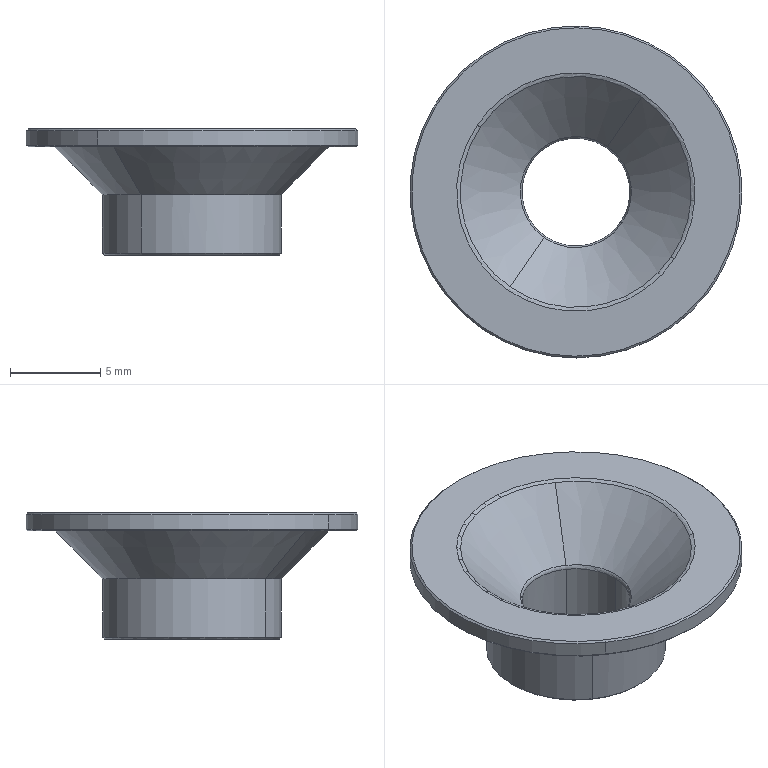Part | SolidWorks | features BaseBody 1 | 1 solid | 30 faces | box 18.44 x 18.44 x 7 mm | volume 502.721 mm3 | cone 14 | cylinder 9 | torus 4 | plane 3 | commonest cylinder face diameters 6 x3 9.94 x3 18.44 x3
STEP:
#1=CARTESIAN_POINT('',(96.116,-202.239,3.349));
#2=VERTEX_POINT('',#1);
#3=CARTESIAN_POINT('',(96.116,-202.239,0.1));
#4=VERTEX_POINT('',#3);
#5=CARTESIAN_POINT('',(96.116,-202.239,2.124));
#6=DIRECTION('',(0.,0.,-1.));
#7=VECTOR('',#6,1000.);
#8=LINE('',#5,#7);
#9=EDGE_CURVE('',#2,#4,#8,.T.);
#10=ORIENTED_EDGE('',*,*,#9,.F.);
#11=CARTESIAN_POINT('',(88.325,-206.142,3.349));
#12=VERTEX_POINT('',#11);
#13=CARTESIAN_POINT('',(91.15,-202.053,3.349));
#14=DIRECTION('',(0.,0.,-1.));
#15=DIRECTION('',(0.5684,0.8228,0.));
#16=AXIS2_PLACEMENT_3D('',#13,#14,#15);
#17=CIRCLE('',#16,4.97);
#18=EDGE_CURVE('',#2,#12,#17,.T.);
#19=ORIENTED_EDGE('',*,*,#18,.T.);
#20=CARTESIAN_POINT('',(88.325,-206.142,0.1));
#21=VERTEX_POINT('',#20);
#22=CARTESIAN_POINT('',(88.325,-206.142,0.1));
#23=DIRECTION('',(0.,0.,1.));
#24=VECTOR('',#23,1000.);
#25=LINE('',#22,#24);
#26=EDGE_CURVE('',#21,#12,#25,.T.);
#27=ORIENTED_EDGE('',*,*,#26,.F.);
#28=CARTESIAN_POINT('',(90.964,-207.019,0.1));
#29=VERTEX_POINT('',#28);
#30=CARTESIAN_POINT('',(91.15,-202.053,0.1));
#31=DIRECTION('',(0.,0.,1.));
#32=DIRECTION('',(-0.5684,-0.8228,0.));
#33=AXIS2_PLACEMENT_3D('',#30,#31,#32);
#34=CIRCLE('',#33,4.97);
#35=EDGE_CURVE('',#21,#29,#34,.T.);
#36=ORIENTED_EDGE('',*,*,#35,.T.);
#37=CARTESIAN_POINT('',(91.15,-202.053,0.1));
#38=DIRECTION('',(0.,0.,1.));
#39=DIRECTION('',(-0.5684,-0.8228,0.));
#40=AXIS2_PLACEMENT_3D('',#37,#38,#39);
#41=CIRCLE('',#40,4.97);
#42=EDGE_CURVE('',#29,#4,#41,.T.);
#43=ORIENTED_EDGE('',*,*,#42,.T.);
#44=EDGE_LOOP('',(#10,#19,#27,#36,#43));
#45=FACE_OUTER_BOUND('',#44,.T.);
#46=CARTESIAN_POINT('',(91.15,-202.053,2.124));
#47=DIRECTION('',(0.,0.,-1.));
#48=DIRECTION('',(0.9993,-0.03741,0.));
#49=AXIS2_PLACEMENT_3D('',#46,#47,#48);
#50=CYLINDRICAL_SURFACE('',#49,4.97);
#51=ADVANCED_FACE('',(#45),#50,.T.);
#52=CARTESIAN_POINT('',(90.967,-206.919,0.));
#53=VERTEX_POINT('',#52);
#54=CARTESIAN_POINT('',(90.966,-206.969,0.05));
#55=DIRECTION('',(-0.02645,-0.7066,0.7071));
#56=VECTOR('',#55,1000.);
#57=LINE('',#54,#56);
#58=EDGE_CURVE('',#53,#29,#57,.T.);
#59=ORIENTED_EDGE('',*,*,#58,.F.);
#60=CARTESIAN_POINT('',(93.918,-198.046,0.));
#61=VERTEX_POINT('',#60);
#62=CARTESIAN_POINT('',(91.15,-202.053,0.));
#63=DIRECTION('',(0.,0.,1.));
#64=DIRECTION('',(-0.5684,-0.8228,0.));
#65=AXIS2_PLACEMENT_3D('',#62,#63,#64);
#66=CIRCLE('',#65,4.87);
#67=EDGE_CURVE('',#53,#61,#66,.T.);
#68=ORIENTED_EDGE('',*,*,#67,.T.);
#69=CARTESIAN_POINT('',(93.974,-197.964,0.1));
#70=VERTEX_POINT('',#69);
#71=CARTESIAN_POINT('',(93.974,-197.964,0.1));
#72=DIRECTION('',(-0.4019,-0.5818,-0.7071));
#73=VECTOR('',#72,1000.);
#74=LINE('',#71,#73);
#75=EDGE_CURVE('',#70,#61,#74,.T.);
#76=ORIENTED_EDGE('',*,*,#75,.F.);
#77=CARTESIAN_POINT('',(91.15,-202.053,0.1));
#78=DIRECTION('',(0.,0.,1.));
#79=DIRECTION('',(-0.5684,-0.8228,0.));
#80=AXIS2_PLACEMENT_3D('',#77,#78,#79);
#81=CIRCLE('',#80,4.97);
#82=EDGE_CURVE('',#4,#70,#81,.T.);
#83=ORIENTED_EDGE('',*,*,#82,.F.);
#84=ORIENTED_EDGE('',*,*,#42,.F.);
#85=EDGE_LOOP('',(#59,#68,#76,#83,#84));
#86=FACE_OUTER_BOUND('',#85,.T.);
#87=CARTESIAN_POINT('',(91.15,-202.053,0.05));
#88=DIRECTION('',(0.,0.,1.));
#89=DIRECTION('',(-0.03741,-0.9993,0.));
#90=AXIS2_PLACEMENT_3D('',#87,#88,#89);
#91=CONICAL_SURFACE('',#90,4.92,0.7854);
#92=ADVANCED_FACE('',(#86),#91,.T.);
#93=ORIENTED_EDGE('',*,*,#75,.T.);
#94=CARTESIAN_POINT('',(88.382,-206.06,0.));
#95=VERTEX_POINT('',#94);
#96=CARTESIAN_POINT('',(91.15,-202.053,0.));
#97=DIRECTION('',(0.,0.,1.));
#98=DIRECTION('',(0.5684,0.8228,0.));
#99=AXIS2_PLACEMENT_3D('',#96,#97,#98);
#100=CIRCLE('',#99,4.87);
#101=EDGE_CURVE('',#61,#95,#100,.T.);
#102=ORIENTED_EDGE('',*,*,#101,.T.);
#103=CARTESIAN_POINT('',(88.325,-206.142,0.1));
#104=DIRECTION('',(0.4019,0.5818,-0.7071));
#105=VECTOR('',#104,1000.);
#106=LINE('',#103,#105);
#107=EDGE_CURVE('',#21,#95,#106,.T.);
#108=ORIENTED_EDGE('',*,*,#107,.F.);
#109=CARTESIAN_POINT('',(91.15,-202.053,0.1));
#110=DIRECTION('',(0.,0.,1.));
#111=DIRECTION('',(-0.9993,0.03741,0.));
#112=AXIS2_PLACEMENT_3D('',#109,#110,#111);
#113=CIRCLE('',#112,4.97);
#114=EDGE_CURVE('',#70,#21,#113,.T.);
#115=ORIENTED_EDGE('',*,*,#114,.F.);
#116=EDGE_LOOP('',(#93,#102,#108,#115));
#117=FACE_OUTER_BOUND('',#116,.T.);
#118=CARTESIAN_POINT('',(91.15,-202.053,0.05));
#119=DIRECTION('',(0.,0.,1.));
#120=DIRECTION('',(-0.03741,-0.9993,0.));
#121=AXIS2_PLACEMENT_3D('',#118,#119,#120);
#122=CONICAL_SURFACE('',#121,4.92,0.7854);
#123=ADVANCED_FACE('',(#117),#122,.T.);
#124=ORIENTED_EDGE('',*,*,#26,.T.);
#125=CARTESIAN_POINT('',(93.974,-197.964,3.349));
#126=VERTEX_POINT('',#125);
#127=CARTESIAN_POINT('',(91.15,-202.053,3.349));
#128=DIRECTION('',(0.,0.,-1.));
#129=DIRECTION('',(-0.5684,-0.8228,0.));
#130=AXIS2_PLACEMENT_3D('',#127,#128,#129);
#131=CIRCLE('',#130,4.97);
#132=EDGE_CURVE('',#12,#126,#131,.T.);
#133=ORIENTED_EDGE('',*,*,#132,.T.);
#134=CARTESIAN_POINT('',(93.974,-197.964,3.349));
#135=DIRECTION('',(0.,0.,-1.));
#136=VECTOR('',#135,1000.);
#137=LINE('',#134,#136);
#138=EDGE_CURVE('',#126,#70,#137,.T.);
#139=ORIENTED_EDGE('',*,*,#138,.T.);
#140=ORIENTED_EDGE('',*,*,#114,.T.);
#141=EDGE_LOOP('',(#124,#133,#139,#140));
#142=FACE_OUTER_BOUND('',#141,.T.);
#143=CARTESIAN_POINT('',(91.15,-202.053,2.124));
#144=DIRECTION('',(0.,0.,-1.));
#145=DIRECTION('',(0.9993,-0.03741,0.));
#146=AXIS2_PLACEMENT_3D('',#143,#144,#145);
#147=CYLINDRICAL_SURFACE('',#146,4.97);
#148=ADVANCED_FACE('',(#142),#147,.T.);
#149=CARTESIAN_POINT('',(86.818,-208.323,6.));
#150=VERTEX_POINT('',#149);
#151=CARTESIAN_POINT('',(88.325,-206.142,3.349));
#152=DIRECTION('',(-0.4019,-0.5818,0.7071));
#153=VECTOR('',#152,1000.);
#154=LINE('',#151,#153);
#155=EDGE_CURVE('',#12,#150,#154,.T.);
#156=ORIENTED_EDGE('',*,*,#155,.T.);
#157=CARTESIAN_POINT('',(95.481,-195.782,6.));
#158=VERTEX_POINT('',#157);
#159=CARTESIAN_POINT('',(91.15,-202.053,6.));
#160=DIRECTION('',(0.,0.,-1.));
#161=DIRECTION('',(-0.5684,-0.8228,0.));
#162=AXIS2_PLACEMENT_3D('',#159,#160,#161);
#163=CIRCLE('',#162,7.621);
#164=EDGE_CURVE('',#150,#158,#163,.T.);
#165=ORIENTED_EDGE('',*,*,#164,.T.);
#166=CARTESIAN_POINT('',(95.481,-195.782,6.));
#167=DIRECTION('',(-0.4019,-0.5818,-0.7071));
#168=VECTOR('',#167,1000.);
#169=LINE('',#166,#168);
#170=EDGE_CURVE('',#158,#126,#169,.T.);
#171=ORIENTED_EDGE('',*,*,#170,.T.);
#172=ORIENTED_EDGE('',*,*,#132,.F.);
#173=EDGE_LOOP('',(#156,#165,#171,#172));
#174=FACE_OUTER_BOUND('',#173,.T.);
#175=CARTESIAN_POINT('',(91.15,-202.053,4.674));
#176=DIRECTION('',(0.,0.,1.));
#177=DIRECTION('',(0.8228,-0.5684,0.));
#178=AXIS2_PLACEMENT_3D('',#175,#176,#177);
#179=CONICAL_SURFACE('',#178,6.296,0.7854);
#180=ADVANCED_FACE('',(#174),#179,.T.);
#181=ORIENTED_EDGE('',*,*,#155,.F.);
#182=ORIENTED_EDGE('',*,*,#18,.F.);
#183=CARTESIAN_POINT('',(91.15,-202.053,3.349));
#184=DIRECTION('',(0.,0.,-1.));
#185=DIRECTION('',(0.5684,0.8228,0.));
#186=AXIS2_PLACEMENT_3D('',#183,#184,#185);
#187=CIRCLE('',#186,4.97);
#188=EDGE_CURVE('',#126,#2,#187,.T.);
#189=ORIENTED_EDGE('',*,*,#188,.F.);
#190=ORIENTED_EDGE('',*,*,#170,.F.);
#191=CARTESIAN_POINT('',(91.15,-202.053,6.));
#192=DIRECTION('',(0.,0.,-1.));
#193=DIRECTION('',(0.5684,0.8228,0.));
#194=AXIS2_PLACEMENT_3D('',#191,#192,#193);
#195=CIRCLE('',#194,7.621);
#196=EDGE_CURVE('',#158,#150,#195,.T.);
#197=ORIENTED_EDGE('',*,*,#196,.T.);
#198=EDGE_LOOP('',(#181,#182,#189,#190,#197));
#199=FACE_OUTER_BOUND('',#198,.T.);
#200=CARTESIAN_POINT('',(91.15,-202.053,4.674));
#201=DIRECTION('',(0.,0.,1.));
#202=DIRECTION('',(-0.8228,0.5684,0.));
#203=AXIS2_PLACEMENT_3D('',#200,#201,#202);
#204=CONICAL_SURFACE('',#203,6.296,0.7854);
#205=ADVANCED_FACE('',(#199),#204,.T.);
#206=ORIENTED_EDGE('',*,*,#164,.F.);
#207=ORIENTED_EDGE('',*,*,#196,.F.);
#208=EDGE_LOOP('',(#206,#207));
#209=FACE_BOUND('',#208,.T.);
#210=CARTESIAN_POINT('',(85.966,-209.556,6.));
#211=VERTEX_POINT('',#210);
#212=CARTESIAN_POINT('',(96.333,-194.549,6.));
#213=VERTEX_POINT('',#212);
#214=CARTESIAN_POINT('',(91.15,-202.053,6.));
#215=DIRECTION('',(0.,0.,1.));
#216=DIRECTION('',(-0.5684,-0.8228,0.));
#217=AXIS2_PLACEMENT_3D('',#214,#215,#216);
#218=CIRCLE('',#217,9.12);
#219=EDGE_CURVE('',#211,#213,#218,.T.);
#220=ORIENTED_EDGE('',*,*,#219,.F.);
#221=CARTESIAN_POINT('',(91.15,-202.053,6.));
#222=DIRECTION('',(0.,0.,1.));
#223=DIRECTION('',(-0.8228,0.5684,0.));
#224=AXIS2_PLACEMENT_3D('',#221,#222,#223);
#225=CIRCLE('',#224,9.12);
#226=EDGE_CURVE('',#213,#211,#225,.T.);
#227=ORIENTED_EDGE('',*,*,#226,.F.);
#228=EDGE_LOOP('',(#220,#227));
#229=FACE_OUTER_BOUND('',#228,.T.);
#230=CARTESIAN_POINT('',(106.374,-199.269,6.));
#231=DIRECTION('',(0.,0.,-1.));
#232=DIRECTION('',(0.,-1.,0.));
#233=AXIS2_PLACEMENT_3D('',#230,#231,#232);
#234=PLANE('',#233);
#235=ADVANCED_FACE('',(#209,#229),#234,.T.);
#236=ORIENTED_EDGE('',*,*,#219,.T.);
#237=CARTESIAN_POINT('',(96.39,-194.467,6.1));
#238=VERTEX_POINT('',#237);
#239=CARTESIAN_POINT('',(96.39,-194.467,6.1));
#240=DIRECTION('',(-0.4019,-0.5818,-0.7071));
#241=VECTOR('',#240,1000.);
#242=LINE('',#239,#241);
#243=EDGE_CURVE('',#238,#213,#242,.T.);
#244=ORIENTED_EDGE('',*,*,#243,.F.);
#245=CARTESIAN_POINT('',(100.363,-202.398,6.1));
#246=VERTEX_POINT('',#245);
#247=CARTESIAN_POINT('',(91.15,-202.053,6.1));
#248=DIRECTION('',(0.,0.,1.));
#249=DIRECTION('',(0.9993,-0.03741,0.));
#250=AXIS2_PLACEMENT_3D('',#247,#248,#249);
#251=CIRCLE('',#250,9.22);
#252=EDGE_CURVE('',#246,#238,#251,.T.);
#253=ORIENTED_EDGE('',*,*,#252,.F.);
#254=CARTESIAN_POINT('',(85.909,-209.639,6.1));
#255=VERTEX_POINT('',#254);
#256=CARTESIAN_POINT('',(91.15,-202.053,6.1));
#257=DIRECTION('',(0.,0.,1.));
#258=DIRECTION('',(0.9993,-0.03741,0.));
#259=AXIS2_PLACEMENT_3D('',#256,#257,#258);
#260=CIRCLE('',#259,9.22);
#261=EDGE_CURVE('',#255,#246,#260,.T.);
#262=ORIENTED_EDGE('',*,*,#261,.F.);
#263=CARTESIAN_POINT('',(85.966,-209.556,6.));
#264=DIRECTION('',(-0.4019,-0.5818,0.7071));
#265=VECTOR('',#264,1000.);
#266=LINE('',#263,#265);
#267=EDGE_CURVE('',#211,#255,#266,.T.);
#268=ORIENTED_EDGE('',*,*,#267,.F.);
#269=EDGE_LOOP('',(#236,#244,#253,#262,#268));
#270=FACE_OUTER_BOUND('',#269,.T.);
#271=CARTESIAN_POINT('',(91.15,-202.053,6.05));
#272=DIRECTION('',(0.,0.,1.));
#273=DIRECTION('',(-0.8228,0.5684,0.));
#274=AXIS2_PLACEMENT_3D('',#271,#272,#273);
#275=CONICAL_SURFACE('',#274,9.17,0.7854);
#276=ADVANCED_FACE('',(#270),#275,.T.);
#277=ORIENTED_EDGE('',*,*,#226,.T.);
#278=ORIENTED_EDGE('',*,*,#267,.T.);
#279=CARTESIAN_POINT('',(91.15,-202.053,6.1));
#280=DIRECTION('',(0.,0.,1.));
#281=DIRECTION('',(-0.9993,0.03741,0.));
#282=AXIS2_PLACEMENT_3D('',#279,#280,#281);
#283=CIRCLE('',#282,9.22);
#284=EDGE_CURVE('',#238,#255,#283,.T.);
#285=ORIENTED_EDGE('',*,*,#284,.F.);
#286=ORIENTED_EDGE('',*,*,#243,.T.);
#287=EDGE_LOOP('',(#277,#278,#285,#286));
#288=FACE_OUTER_BOUND('',#287,.T.);
#289=CARTESIAN_POINT('',(91.15,-202.053,6.05));
#290=DIRECTION('',(0.,0.,1.));
#291=DIRECTION('',(0.8228,-0.5684,0.));
#292=AXIS2_PLACEMENT_3D('',#289,#290,#291);
#293=CONICAL_SURFACE('',#292,9.17,0.7854);
#294=ADVANCED_FACE('',(#288),#293,.T.);
#295=CARTESIAN_POINT('',(85.909,-209.639,6.9));
#296=VERTEX_POINT('',#295);
#297=CARTESIAN_POINT('',(96.39,-194.467,6.9));
#298=VERTEX_POINT('',#297);
#299=CARTESIAN_POINT('',(91.15,-202.053,6.9));
#300=DIRECTION('',(0.,0.,-1.));
#301=DIRECTION('',(-0.9993,0.03741,0.));
#302=AXIS2_PLACEMENT_3D('',#299,#300,#301);
#303=CIRCLE('',#302,9.22);
#304=EDGE_CURVE('',#296,#298,#303,.T.);
#305=ORIENTED_EDGE('',*,*,#304,.T.);
#306=CARTESIAN_POINT('',(96.39,-194.467,6.9));
#307=DIRECTION('',(0.,0.,-1.));
#308=VECTOR('',#307,1000.);
#309=LINE('',#306,#308);
#310=EDGE_CURVE('',#298,#238,#309,.T.);
#311=ORIENTED_EDGE('',*,*,#310,.T.);
#312=ORIENTED_EDGE('',*,*,#284,.T.);
#313=CARTESIAN_POINT('',(85.909,-209.639,6.1));
#314=DIRECTION('',(0.,0.,1.));
#315=VECTOR('',#314,1000.);
#316=LINE('',#313,#315);
#317=EDGE_CURVE('',#255,#296,#316,.T.);
#318=ORIENTED_EDGE('',*,*,#317,.T.);
#319=EDGE_LOOP('',(#305,#311,#312,#318));
#320=FACE_OUTER_BOUND('',#319,.T.);
#321=CARTESIAN_POINT('',(91.15,-202.053,6.5));
#322=DIRECTION('',(0.,0.,-1.));
#323=DIRECTION('',(0.9993,-0.03741,0.));
#324=AXIS2_PLACEMENT_3D('',#321,#322,#323);
#325=CYLINDRICAL_SURFACE('',#324,9.22);
#326=ADVANCED_FACE('',(#320),#325,.T.);
#327=CARTESIAN_POINT('',(85.966,-209.556,7.));
#328=VERTEX_POINT('',#327);
#329=CARTESIAN_POINT('',(96.333,-194.549,7.));
#330=VERTEX_POINT('',#329);
#331=CARTESIAN_POINT('',(91.15,-202.053,7.));
#332=DIRECTION('',(0.,0.,-1.));
#333=DIRECTION('',(-0.8228,0.5684,0.));
#334=AXIS2_PLACEMENT_3D('',#331,#332,#333);
#335=CIRCLE('',#334,9.12);
#336=EDGE_CURVE('',#328,#330,#335,.T.);
#337=ORIENTED_EDGE('',*,*,#336,.T.);
#338=CARTESIAN_POINT('',(96.333,-194.549,7.));
#339=DIRECTION('',(0.4019,0.5818,-0.7071));
#340=VECTOR('',#339,1000.);
#341=LINE('',#338,#340);
#342=EDGE_CURVE('',#330,#298,#341,.T.);
#343=ORIENTED_EDGE('',*,*,#342,.T.);
#344=ORIENTED_EDGE('',*,*,#304,.F.);
#345=CARTESIAN_POINT('',(85.909,-209.639,6.9));
#346=DIRECTION('',(0.4019,0.5818,0.7071));
#347=VECTOR('',#346,1000.);
#348=LINE('',#345,#347);
#349=EDGE_CURVE('',#296,#328,#348,.T.);
#350=ORIENTED_EDGE('',*,*,#349,.T.);
#351=EDGE_LOOP('',(#337,#343,#344,#350));
#352=FACE_OUTER_BOUND('',#351,.T.);
#353=CARTESIAN_POINT('',(91.15,-202.053,6.95));
#354=DIRECTION('',(0.,0.,-1.));
#355=DIRECTION('',(0.8228,-0.5684,0.));
#356=AXIS2_PLACEMENT_3D('',#353,#354,#355);
#357=CONICAL_SURFACE('',#356,9.17,0.7854);
#358=ADVANCED_FACE('',(#352),#357,.T.);
#359=CARTESIAN_POINT('',(85.667,-198.335,7.));
#360=VERTEX_POINT('',#359);
#361=CARTESIAN_POINT('',(96.633,-205.77,7.));
#362=VERTEX_POINT('',#361);
#363=CARTESIAN_POINT('',(91.15,-202.053,7.));
#364=DIRECTION('',(0.,0.,1.));
#365=DIRECTION('',(0.8228,-0.5684,0.));
#366=AXIS2_PLACEMENT_3D('',#363,#364,#365);
#367=CIRCLE('',#366,6.624);
#368=EDGE_CURVE('',#360,#362,#367,.T.);
#369=ORIENTED_EDGE('',*,*,#368,.F.);
#370=CARTESIAN_POINT('',(91.15,-202.053,7.));
#371=DIRECTION('',(0.,0.,1.));
#372=DIRECTION('',(-0.8228,0.5684,0.));
#373=AXIS2_PLACEMENT_3D('',#370,#371,#372);
#374=CIRCLE('',#373,6.624);
#375=EDGE_CURVE('',#362,#360,#374,.T.);
#376=ORIENTED_EDGE('',*,*,#375,.F.);
#377=EDGE_LOOP('',(#369,#376));
#378=FACE_BOUND('',#377,.T.);
#379=ORIENTED_EDGE('',*,*,#336,.F.);
#380=CARTESIAN_POINT('',(91.15,-202.053,7.));
#381=DIRECTION('',(0.,0.,-1.));
#382=DIRECTION('',(0.8228,-0.5684,0.));
#383=AXIS2_PLACEMENT_3D('',#380,#381,#382);
#384=CIRCLE('',#383,9.12);
#385=EDGE_CURVE('',#330,#328,#384,.T.);
#386=ORIENTED_EDGE('',*,*,#385,.F.);
#387=EDGE_LOOP('',(#379,#386));
#388=FACE_OUTER_BOUND('',#387,.T.);
#389=CARTESIAN_POINT('',(109.151,-195.249,7.));
#390=DIRECTION('',(0.,0.,1.));
#391=DIRECTION('',(1.,0.,0.));
#392=AXIS2_PLACEMENT_3D('',#389,#390,#391);
#393=PLANE('',#392);
#394=ADVANCED_FACE('',(#378,#388),#393,.T.);
#395=ORIENTED_EDGE('',*,*,#342,.F.);
#396=ORIENTED_EDGE('',*,*,#385,.T.);
#397=ORIENTED_EDGE('',*,*,#349,.F.);
#398=CARTESIAN_POINT('',(100.363,-202.398,6.9));
#399=VERTEX_POINT('',#398);
#400=CARTESIAN_POINT('',(91.15,-202.053,6.9));
#401=DIRECTION('',(0.,0.,-1.));
#402=DIRECTION('',(0.8228,-0.5684,0.));
#403=AXIS2_PLACEMENT_3D('',#400,#401,#402);
#404=CIRCLE('',#403,9.22);
#405=EDGE_CURVE('',#399,#296,#404,.T.);
#406=ORIENTED_EDGE('',*,*,#405,.F.);
#407=CARTESIAN_POINT('',(91.15,-202.053,6.9));
#408=DIRECTION('',(0.,0.,-1.));
#409=DIRECTION('',(0.8228,-0.5684,0.));
#410=AXIS2_PLACEMENT_3D('',#407,#408,#409);
#411=CIRCLE('',#410,9.22);
#412=EDGE_CURVE('',#298,#399,#411,.T.);
#413=ORIENTED_EDGE('',*,*,#412,.F.);
#414=EDGE_LOOP('',(#395,#396,#397,#406,#413));
#415=FACE_OUTER_BOUND('',#414,.T.);
#416=CARTESIAN_POINT('',(91.15,-202.053,6.95));
#417=DIRECTION('',(0.,0.,-1.));
#418=DIRECTION('',(-0.8228,0.5684,0.));
#419=AXIS2_PLACEMENT_3D('',#416,#417,#418);
#420=CONICAL_SURFACE('',#419,9.17,0.7854);
#421=ADVANCED_FACE('',(#415),#420,.T.);
#422=CARTESIAN_POINT('',(100.363,-202.398,6.5));
#423=DIRECTION('',(0.,0.,-1.));
#424=VECTOR('',#423,1000.);
#425=LINE('',#422,#424);
#426=EDGE_CURVE('',#399,#246,#425,.T.);
#427=ORIENTED_EDGE('',*,*,#426,.F.);
#428=ORIENTED_EDGE('',*,*,#405,.T.);
#429=ORIENTED_EDGE('',*,*,#317,.F.);
#430=ORIENTED_EDGE('',*,*,#261,.T.);
#431=EDGE_LOOP('',(#427,#428,#429,#430));
#432=FACE_OUTER_BOUND('',#431,.T.);
#433=CARTESIAN_POINT('',(91.15,-202.053,6.5));
#434=DIRECTION('',(0.,0.,-1.));
#435=DIRECTION('',(0.9993,-0.03741,0.));
#436=AXIS2_PLACEMENT_3D('',#433,#434,#435);
#437=CYLINDRICAL_SURFACE('',#436,9.22);
#438=ADVANCED_FACE('',(#432),#437,.T.);
#439=CARTESIAN_POINT('',(96.457,-205.651,6.912));
#440=VERTEX_POINT('',#439);
#441=CARTESIAN_POINT('',(96.633,-205.77,6.7));
#442=DIRECTION('',(-0.5612,-0.8277,0.));
#443=DIRECTION('',(0.000000292,-0.000000198,1.));
#444=AXIS2_PLACEMENT_3D('',#441,#442,#443);
#445=CIRCLE('',#444,0.3);
#446=EDGE_CURVE('',#362,#440,#445,.T.);
#447=ORIENTED_EDGE('',*,*,#446,.F.);
#448=ORIENTED_EDGE('',*,*,#375,.T.);
#449=CARTESIAN_POINT('',(85.842,-198.455,6.912));
#450=VERTEX_POINT('',#449);
#451=CARTESIAN_POINT('',(85.667,-198.335,6.7));
#452=DIRECTION('',(-0.5612,-0.8277,0.));
#453=DIRECTION('',(0.5853,-0.3968,0.7071));
#454=AXIS2_PLACEMENT_3D('',#451,#452,#453);
#455=CIRCLE('',#454,0.3);
#456=EDGE_CURVE('',#450,#360,#455,.T.);
#457=ORIENTED_EDGE('',*,*,#456,.F.);
#458=CARTESIAN_POINT('',(85.874,-198.408,6.912));
#459=VERTEX_POINT('',#458);
#460=CARTESIAN_POINT('',(91.15,-202.053,6.912));
#461=DIRECTION('',(0.,0.,1.));
#462=DIRECTION('',(-0.8228,0.5684,0.));
#463=AXIS2_PLACEMENT_3D('',#460,#461,#462);
#464=CIRCLE('',#463,6.412);
#465=EDGE_CURVE('',#459,#450,#464,.T.);
#466=ORIENTED_EDGE('',*,*,#465,.F.);
#467=CARTESIAN_POINT('',(94.794,-196.777,6.912));
#468=VERTEX_POINT('',#467);
#469=CARTESIAN_POINT('',(91.15,-202.053,6.912));
#470=DIRECTION('',(0.,0.,1.));
#471=DIRECTION('',(0.5684,0.8228,0.));
#472=AXIS2_PLACEMENT_3D('',#469,#470,#471);
#473=CIRCLE('',#472,6.412);
#474=EDGE_CURVE('',#468,#459,#473,.T.);
#475=ORIENTED_EDGE('',*,*,#474,.F.);
#476=CARTESIAN_POINT('',(91.15,-202.053,6.912));
#477=DIRECTION('',(0.,0.,1.));
#478=DIRECTION('',(0.8277,-0.5612,0.));
#479=AXIS2_PLACEMENT_3D('',#476,#477,#478);
#480=CIRCLE('',#479,6.412);
#481=EDGE_CURVE('',#440,#468,#480,.T.);
#482=ORIENTED_EDGE('',*,*,#481,.F.);
#483=EDGE_LOOP('',(#447,#448,#457,#466,#475,#482));
#484=FACE_OUTER_BOUND('',#483,.T.);
#485=CARTESIAN_POINT('',(91.15,-202.053,6.7));
#486=DIRECTION('',(0.,0.,-1.));
#487=DIRECTION('',(-0.8277,0.5612,0.));
#488=AXIS2_PLACEMENT_3D('',#485,#486,#487);
#489=TOROIDAL_SURFACE('',#488,6.624,0.3);
#490=ADVANCED_FACE('',(#484),#489,.T.);
#491=ORIENTED_EDGE('',*,*,#446,.T.);
#492=CARTESIAN_POINT('',(96.425,-205.697,6.912));
#493=VERTEX_POINT('',#492);
#494=CARTESIAN_POINT('',(91.15,-202.053,6.912));
#495=DIRECTION('',(0.,0.,1.));
#496=DIRECTION('',(0.8228,-0.5684,0.));
#497=AXIS2_PLACEMENT_3D('',#494,#495,#496);
#498=CIRCLE('',#497,6.412);
#499=EDGE_CURVE('',#493,#440,#498,.T.);
#500=ORIENTED_EDGE('',*,*,#499,.F.);
#501=CARTESIAN_POINT('',(87.505,-207.329,6.912));
#502=VERTEX_POINT('',#501);
#503=CARTESIAN_POINT('',(91.15,-202.053,6.912));
#504=DIRECTION('',(0.,0.,1.));
#505=DIRECTION('',(-0.5684,-0.8228,0.));
#506=AXIS2_PLACEMENT_3D('',#503,#504,#505);
#507=CIRCLE('',#506,6.412);
#508=EDGE_CURVE('',#502,#493,#507,.T.);
#509=ORIENTED_EDGE('',*,*,#508,.F.);
#510=CARTESIAN_POINT('',(91.15,-202.053,6.912));
#511=DIRECTION('',(0.,0.,1.));
#512=DIRECTION('',(-0.8277,0.5612,0.));
#513=AXIS2_PLACEMENT_3D('',#510,#511,#512);
#514=CIRCLE('',#513,6.412);
#515=EDGE_CURVE('',#450,#502,#514,.T.);
#516=ORIENTED_EDGE('',*,*,#515,.F.);
#517=ORIENTED_EDGE('',*,*,#456,.T.);
#518=ORIENTED_EDGE('',*,*,#368,.T.);
#519=EDGE_LOOP('',(#491,#500,#509,#516,#517,#518));
#520=FACE_OUTER_BOUND('',#519,.T.);
#521=CARTESIAN_POINT('',(91.15,-202.053,6.7));
#522=DIRECTION('',(0.,0.,-1.));
#523=DIRECTION('',(0.8277,-0.5612,0.));
#524=AXIS2_PLACEMENT_3D('',#521,#522,#523);
#525=TOROIDAL_SURFACE('',#524,6.624,0.3);
#526=ADVANCED_FACE('',(#520),#525,.T.);
#527=CARTESIAN_POINT('',(88.593,-200.321,3.588));
#528=VERTEX_POINT('',#527);
#529=CARTESIAN_POINT('',(88.609,-200.298,3.588));
#530=VERTEX_POINT('',#529);
#531=CARTESIAN_POINT('',(91.15,-202.053,3.588));
#532=DIRECTION('',(0.,0.,-1.));
#533=DIRECTION('',(-0.8279,0.5608,0.));
#534=AXIS2_PLACEMENT_3D('',#531,#532,#533);
#535=CIRCLE('',#534,3.088);
#536=EDGE_CURVE('',#528,#530,#535,.T.);
#537=ORIENTED_EDGE('',*,*,#536,.T.);
#538=CARTESIAN_POINT('',(92.905,-199.512,3.588));
#539=VERTEX_POINT('',#538);
#540=CARTESIAN_POINT('',(91.15,-202.053,3.588));
#541=DIRECTION('',(0.,0.,-1.));
#542=DIRECTION('',(-0.8228,0.5684,0.));
#543=AXIS2_PLACEMENT_3D('',#540,#541,#542);
#544=CIRCLE('',#543,3.088);
#545=EDGE_CURVE('',#530,#539,#544,.T.);
#546=ORIENTED_EDGE('',*,*,#545,.T.);
#547=CARTESIAN_POINT('',(92.905,-199.512,3.588));
#548=DIRECTION('',(0.4019,0.5818,0.7071));
#549=VECTOR('',#548,1000.);
#550=LINE('',#547,#549);
#551=EDGE_CURVE('',#539,#468,#550,.T.);
#552=ORIENTED_EDGE('',*,*,#551,.T.);
#553=ORIENTED_EDGE('',*,*,#474,.T.);
#554=ORIENTED_EDGE('',*,*,#465,.T.);
#555=ORIENTED_EDGE('',*,*,#515,.T.);
#556=CARTESIAN_POINT('',(89.395,-204.593,3.588));
#557=VERTEX_POINT('',#556);
#558=CARTESIAN_POINT('',(87.505,-207.329,6.912));
#559=DIRECTION('',(0.4019,0.5818,-0.7071));
#560=VECTOR('',#559,1000.);
#561=LINE('',#558,#560);
#562=EDGE_CURVE('',#502,#557,#561,.T.);
#563=ORIENTED_EDGE('',*,*,#562,.T.);
#564=CARTESIAN_POINT('',(91.15,-202.053,3.588));
#565=DIRECTION('',(0.,0.,-1.));
#566=DIRECTION('',(-0.5684,-0.8228,0.));
#567=AXIS2_PLACEMENT_3D('',#564,#565,#566);
#568=CIRCLE('',#567,3.088);
#569=EDGE_CURVE('',#557,#528,#568,.T.);
#570=ORIENTED_EDGE('',*,*,#569,.T.);
#571=EDGE_LOOP('',(#537,#546,#552,#553,#554,#555,#563,#570));
#572=FACE_OUTER_BOUND('',#571,.T.);
#573=CARTESIAN_POINT('',(91.15,-202.053,5.25));
#574=DIRECTION('',(0.,0.,1.));
#575=DIRECTION('',(0.5684,0.8228,0.));
#576=AXIS2_PLACEMENT_3D('',#573,#574,#575);
#577=CONICAL_SURFACE('',#576,4.75,0.7854);
#578=ADVANCED_FACE('',(#572),#577,.F.);
#579=CARTESIAN_POINT('',(89.445,-204.521,3.376));
#580=VERTEX_POINT('',#579);
#581=CARTESIAN_POINT('',(93.633,-203.735,3.376));
#582=VERTEX_POINT('',#581);
#583=CARTESIAN_POINT('',(91.15,-202.053,3.376));
#584=DIRECTION('',(0.,0.,1.));
#585=DIRECTION('',(-0.5684,-0.8228,0.));
#586=AXIS2_PLACEMENT_3D('',#583,#584,#585);
#587=CIRCLE('',#586,3.);
#588=EDGE_CURVE('',#580,#582,#587,.T.);
#589=ORIENTED_EDGE('',*,*,#588,.F.);
#590=CARTESIAN_POINT('',(88.666,-200.37,3.376));
#591=VERTEX_POINT('',#590);
#592=CARTESIAN_POINT('',(91.15,-202.053,3.376));
#593=DIRECTION('',(0.,0.,1.));
#594=DIRECTION('',(-0.9993,0.03741,0.));
#595=AXIS2_PLACEMENT_3D('',#592,#593,#594);
#596=CIRCLE('',#595,3.);
#597=EDGE_CURVE('',#591,#580,#596,.T.);
#598=ORIENTED_EDGE('',*,*,#597,.F.);
#599=CARTESIAN_POINT('',(88.417,-200.202,3.376));
#600=DIRECTION('',(-0.5608,-0.8279,0.));
#601=DIRECTION('',(0.8279,-0.5608,0.));
#602=AXIS2_PLACEMENT_3D('',#599,#600,#601);
#603=CIRCLE('',#602,0.3);
#604=EDGE_CURVE('',#591,#528,#603,.T.);
#605=ORIENTED_EDGE('',*,*,#604,.T.);
#606=ORIENTED_EDGE('',*,*,#569,.F.);
#607=CARTESIAN_POINT('',(93.69,-203.808,3.588));
#608=VERTEX_POINT('',#607);
#609=CARTESIAN_POINT('',(91.15,-202.053,3.588));
#610=DIRECTION('',(0.,0.,-1.));
#611=DIRECTION('',(0.8228,-0.5684,0.));
#612=AXIS2_PLACEMENT_3D('',#609,#610,#611);
#613=CIRCLE('',#612,3.088);
#614=EDGE_CURVE('',#608,#557,#613,.T.);
#615=ORIENTED_EDGE('',*,*,#614,.F.);
#616=CARTESIAN_POINT('',(93.706,-203.785,3.588));
#617=VERTEX_POINT('',#616);
#618=CARTESIAN_POINT('',(91.15,-202.053,3.588));
#619=DIRECTION('',(0.,0.,-1.));
#620=DIRECTION('',(0.828,-0.5608,0.));
#621=AXIS2_PLACEMENT_3D('',#618,#619,#620);
#622=CIRCLE('',#621,3.088);
#623=EDGE_CURVE('',#617,#608,#622,.T.);
#624=ORIENTED_EDGE('',*,*,#623,.F.);
#625=CARTESIAN_POINT('',(93.882,-203.904,3.376));
#626=DIRECTION('',(-0.5608,-0.8279,0.));
#627=DIRECTION('',(-0.5855,0.3966,0.7071));
#628=AXIS2_PLACEMENT_3D('',#625,#626,#627);
#629=CIRCLE('',#628,0.3);
#630=EDGE_CURVE('',#617,#582,#629,.T.);
#631=ORIENTED_EDGE('',*,*,#630,.T.);
#632=EDGE_LOOP('',(#589,#598,#605,#606,#615,#624,#631));
#633=FACE_OUTER_BOUND('',#632,.T.);
#634=CARTESIAN_POINT('',(91.15,-202.053,3.376));
#635=DIRECTION('',(0.,0.,-1.));
#636=DIRECTION('',(0.8279,-0.5608,0.));
#637=AXIS2_PLACEMENT_3D('',#634,#635,#636);
#638=TOROIDAL_SURFACE('',#637,3.3,0.3);
#639=ADVANCED_FACE('',(#633),#638,.T.);
#640=CARTESIAN_POINT('',(92.855,-199.584,3.376));
#641=VERTEX_POINT('',#640);
#642=CARTESIAN_POINT('',(91.15,-202.053,3.376));
#643=DIRECTION('',(0.,0.,1.));
#644=DIRECTION('',(0.5684,0.8228,0.));
#645=AXIS2_PLACEMENT_3D('',#642,#643,#644);
#646=CIRCLE('',#645,3.);
#647=EDGE_CURVE('',#641,#591,#646,.T.);
#648=ORIENTED_EDGE('',*,*,#647,.F.);
#649=CARTESIAN_POINT('',(94.148,-202.165,3.376));
#650=VERTEX_POINT('',#649);
#651=CARTESIAN_POINT('',(91.15,-202.053,3.376));
#652=DIRECTION('',(0.,0.,1.));
#653=DIRECTION('',(0.9993,-0.03741,0.));
#654=AXIS2_PLACEMENT_3D('',#651,#652,#653);
#655=CIRCLE('',#654,3.);
#656=EDGE_CURVE('',#650,#641,#655,.T.);
#657=ORIENTED_EDGE('',*,*,#656,.F.);
#658=CARTESIAN_POINT('',(91.15,-202.053,3.376));
#659=DIRECTION('',(0.,0.,1.));
#660=DIRECTION('',(0.9993,-0.03741,0.));
#661=AXIS2_PLACEMENT_3D('',#658,#659,#660);
#662=CIRCLE('',#661,3.);
#663=EDGE_CURVE('',#582,#650,#662,.T.);
#664=ORIENTED_EDGE('',*,*,#663,.F.);
#665=ORIENTED_EDGE('',*,*,#630,.F.);
#666=CARTESIAN_POINT('',(91.15,-202.053,3.588));
#667=DIRECTION('',(0.,0.,-1.));
#668=DIRECTION('',(0.5684,0.8228,0.));
#669=AXIS2_PLACEMENT_3D('',#666,#667,#668);
#670=CIRCLE('',#669,3.088);
#671=EDGE_CURVE('',#539,#617,#670,.T.);
#672=ORIENTED_EDGE('',*,*,#671,.F.);
#673=ORIENTED_EDGE('',*,*,#545,.F.);
#674=ORIENTED_EDGE('',*,*,#536,.F.);
#675=ORIENTED_EDGE('',*,*,#604,.F.);
#676=EDGE_LOOP('',(#648,#657,#664,#665,#672,#673,#674,#675));
#677=FACE_OUTER_BOUND('',#676,.T.);
#678=CARTESIAN_POINT('',(91.15,-202.053,3.376));
#679=DIRECTION('',(0.,0.,-1.));
#680=DIRECTION('',(-0.8279,0.5608,0.));
#681=AXIS2_PLACEMENT_3D('',#678,#679,#680);
#682=TOROIDAL_SURFACE('',#681,3.3,0.3);
#683=ADVANCED_FACE('',(#677),#682,.T.);
#684=ORIENTED_EDGE('',*,*,#508,.T.);
#685=ORIENTED_EDGE('',*,*,#499,.T.);
#686=ORIENTED_EDGE('',*,*,#481,.T.);
#687=ORIENTED_EDGE('',*,*,#551,.F.);
#688=ORIENTED_EDGE('',*,*,#671,.T.);
#689=ORIENTED_EDGE('',*,*,#623,.T.);
#690=ORIENTED_EDGE('',*,*,#614,.T.);
#691=ORIENTED_EDGE('',*,*,#562,.F.);
#692=EDGE_LOOP('',(#684,#685,#686,#687,#688,#689,#690,#691));
#693=FACE_OUTER_BOUND('',#692,.T.);
#694=CARTESIAN_POINT('',(91.15,-202.053,5.25));
#695=DIRECTION('',(0.,0.,1.));
#696=DIRECTION('',(-0.5684,-0.8228,0.));
#697=AXIS2_PLACEMENT_3D('',#694,#695,#696);
#698=CONICAL_SURFACE('',#697,4.75,0.7854);
#699=ADVANCED_FACE('',(#693),#698,.F.);
#700=CARTESIAN_POINT('',(94.148,-202.165,0.1));
#701=VERTEX_POINT('',#700);
#702=CARTESIAN_POINT('',(94.148,-202.165,1.888));
#703=DIRECTION('',(0.,0.,-1.));
#704=VECTOR('',#703,1000.);
#705=LINE('',#702,#704);
#706=EDGE_CURVE('',#650,#701,#705,.T.);
#707=ORIENTED_EDGE('',*,*,#706,.F.);
#708=ORIENTED_EDGE('',*,*,#656,.T.);
#709=CARTESIAN_POINT('',(92.855,-199.584,0.1));
#710=VERTEX_POINT('',#709);
#711=CARTESIAN_POINT('',(92.855,-199.584,0.1));
#712=DIRECTION('',(0.,0.,1.));
#713=VECTOR('',#712,1000.);
#714=LINE('',#711,#713);
#715=EDGE_CURVE('',#710,#641,#714,.T.);
#716=ORIENTED_EDGE('',*,*,#715,.F.);
#717=CARTESIAN_POINT('',(91.15,-202.053,0.1));
#718=DIRECTION('',(0.,0.,-1.));
#719=DIRECTION('',(0.5684,0.8228,0.));
#720=AXIS2_PLACEMENT_3D('',#717,#718,#719);
#721=CIRCLE('',#720,3.);
#722=EDGE_CURVE('',#710,#701,#721,.T.);
#723=ORIENTED_EDGE('',*,*,#722,.T.);
#724=EDGE_LOOP('',(#707,#708,#716,#723));
#725=FACE_OUTER_BOUND('',#724,.T.);
#726=CARTESIAN_POINT('',(91.15,-202.053,1.888));
#727=DIRECTION('',(0.,0.,-1.));
#728=DIRECTION('',(0.9993,-0.03741,0.));
#729=AXIS2_PLACEMENT_3D('',#726,#727,#728);
#730=CYLINDRICAL_SURFACE('',#729,3.);
#731=ADVANCED_FACE('',(#725),#730,.F.);
#732=CARTESIAN_POINT('',(91.037,-205.051,0.1));
#733=VERTEX_POINT('',#732);
#734=CARTESIAN_POINT('',(91.034,-205.151,0.));
#735=VERTEX_POINT('',#734);
#736=CARTESIAN_POINT('',(91.036,-205.101,0.05));
#737=DIRECTION('',(-0.02645,-0.7066,-0.7071));
#738=VECTOR('',#737,1000.);
#739=LINE('',#736,#738);
#740=EDGE_CURVE('',#733,#735,#739,.T.);
#741=ORIENTED_EDGE('',*,*,#740,.F.);
#742=CARTESIAN_POINT('',(91.15,-202.053,0.1));
#743=DIRECTION('',(0.,0.,-1.));
#744=DIRECTION('',(0.5684,0.8228,0.));
#745=AXIS2_PLACEMENT_3D('',#742,#743,#744);
#746=CIRCLE('',#745,3.);
#747=EDGE_CURVE('',#701,#733,#746,.T.);
#748=ORIENTED_EDGE('',*,*,#747,.F.);
#749=ORIENTED_EDGE('',*,*,#722,.F.);
#750=CARTESIAN_POINT('',(92.912,-199.502,0.));
#751=VERTEX_POINT('',#750);
#752=CARTESIAN_POINT('',(92.912,-199.502,0.));
#753=DIRECTION('',(-0.4019,-0.5818,0.7071));
#754=VECTOR('',#753,1000.);
#755=LINE('',#752,#754);
#756=EDGE_CURVE('',#751,#710,#755,.T.);
#757=ORIENTED_EDGE('',*,*,#756,.F.);
#758=CARTESIAN_POINT('',(91.15,-202.053,0.));
#759=DIRECTION('',(0.,0.,-1.));
#760=DIRECTION('',(0.5684,0.8228,0.));
#761=AXIS2_PLACEMENT_3D('',#758,#759,#760);
#762=CIRCLE('',#761,3.1);
#763=EDGE_CURVE('',#751,#735,#762,.T.);
#764=ORIENTED_EDGE('',*,*,#763,.T.);
#765=EDGE_LOOP('',(#741,#748,#749,#757,#764));
#766=FACE_OUTER_BOUND('',#765,.T.);
#767=CARTESIAN_POINT('',(91.15,-202.053,0.05));
#768=DIRECTION('',(0.,0.,-1.));
#769=DIRECTION('',(-0.03741,-0.9993,0.));
#770=AXIS2_PLACEMENT_3D('',#767,#768,#769);
#771=CONICAL_SURFACE('',#770,3.05,0.7854);
#772=ADVANCED_FACE('',(#766),#771,.F.);
#773=CARTESIAN_POINT('',(89.388,-204.603,0.));
#774=VERTEX_POINT('',#773);
#775=CARTESIAN_POINT('',(91.15,-202.053,0.));
#776=DIRECTION('',(0.,0.,-1.));
#777=DIRECTION('',(0.03741,0.9993,0.));
#778=AXIS2_PLACEMENT_3D('',#775,#776,#777);
#779=CIRCLE('',#778,3.1);
#780=EDGE_CURVE('',#774,#751,#779,.T.);
#781=ORIENTED_EDGE('',*,*,#780,.F.);
#782=CARTESIAN_POINT('',(91.15,-202.053,0.));
#783=DIRECTION('',(0.,0.,-1.));
#784=DIRECTION('',(0.5684,0.8228,0.));
#785=AXIS2_PLACEMENT_3D('',#782,#783,#784);
#786=CIRCLE('',#785,3.1);
#787=EDGE_CURVE('',#735,#774,#786,.T.);
#788=ORIENTED_EDGE('',*,*,#787,.F.);
#789=ORIENTED_EDGE('',*,*,#763,.F.);
#790=EDGE_LOOP('',(#781,#788,#789));
#791=FACE_BOUND('',#790,.T.);
#792=CARTESIAN_POINT('',(91.15,-202.053,0.));
#793=DIRECTION('',(0.,0.,1.));
#794=DIRECTION('',(-0.5684,-0.8228,0.));
#795=AXIS2_PLACEMENT_3D('',#792,#793,#794);
#796=CIRCLE('',#795,4.87);
#797=EDGE_CURVE('',#95,#53,#796,.T.);
#798=ORIENTED_EDGE('',*,*,#797,.F.);
#799=ORIENTED_EDGE('',*,*,#101,.F.);
#800=ORIENTED_EDGE('',*,*,#67,.F.);
#801=EDGE_LOOP('',(#798,#799,#800));
#802=FACE_OUTER_BOUND('',#801,.T.);
#803=CARTESIAN_POINT('',(100.114,-200.413,0.));
#804=DIRECTION('',(0.,0.,-1.));
#805=DIRECTION('',(0.,-1.,0.));
#806=AXIS2_PLACEMENT_3D('',#803,#804,#805);
#807=PLANE('',#806);
#808=ADVANCED_FACE('',(#791,#802),#807,.T.);
#809=ORIENTED_EDGE('',*,*,#756,.T.);
#810=CARTESIAN_POINT('',(89.445,-204.521,0.1));
#811=VERTEX_POINT('',#810);
#812=CARTESIAN_POINT('',(91.15,-202.053,0.1));
#813=DIRECTION('',(0.,0.,-1.));
#814=DIRECTION('',(0.03741,0.9993,0.));
#815=AXIS2_PLACEMENT_3D('',#812,#813,#814);
#816=CIRCLE('',#815,3.);
#817=EDGE_CURVE('',#811,#710,#816,.T.);
#818=ORIENTED_EDGE('',*,*,#817,.F.);
#819=CARTESIAN_POINT('',(89.388,-204.603,0.));
#820=DIRECTION('',(0.4019,0.5818,0.7071));
#821=VECTOR('',#820,1000.);
#822=LINE('',#819,#821);
#823=EDGE_CURVE('',#774,#811,#822,.T.);
#824=ORIENTED_EDGE('',*,*,#823,.F.);
#825=ORIENTED_EDGE('',*,*,#780,.T.);
#826=EDGE_LOOP('',(#809,#818,#824,#825));
#827=FACE_OUTER_BOUND('',#826,.T.);
#828=CARTESIAN_POINT('',(91.15,-202.053,0.05));
#829=DIRECTION('',(0.,0.,-1.));
#830=DIRECTION('',(-0.03741,-0.9993,0.));
#831=AXIS2_PLACEMENT_3D('',#828,#829,#830);
#832=CONICAL_SURFACE('',#831,3.05,0.7854);
#833=ADVANCED_FACE('',(#827),#832,.F.);
#834=ORIENTED_EDGE('',*,*,#715,.T.);
#835=ORIENTED_EDGE('',*,*,#647,.T.);
#836=ORIENTED_EDGE('',*,*,#597,.T.);
#837=CARTESIAN_POINT('',(89.445,-204.521,3.376));
#838=DIRECTION('',(0.,0.,-1.));
#839=VECTOR('',#838,1000.);
#840=LINE('',#837,#839);
#841=EDGE_CURVE('',#580,#811,#840,.T.);
#842=ORIENTED_EDGE('',*,*,#841,.T.);
#843=ORIENTED_EDGE('',*,*,#817,.T.);
#844=EDGE_LOOP('',(#834,#835,#836,#842,#843));
#845=FACE_OUTER_BOUND('',#844,.T.);
#846=CARTESIAN_POINT('',(91.15,-202.053,1.888));
#847=DIRECTION('',(0.,0.,-1.));
#848=DIRECTION('',(0.9993,-0.03741,0.));
#849=AXIS2_PLACEMENT_3D('',#846,#847,#848);
#850=CYLINDRICAL_SURFACE('',#849,3.);
#851=ADVANCED_FACE('',(#845),#850,.F.);
#852=CARTESIAN_POINT('',(91.15,-202.053,0.1));
#853=DIRECTION('',(0.,0.,-1.));
#854=DIRECTION('',(0.5684,0.8228,0.));
#855=AXIS2_PLACEMENT_3D('',#852,#853,#854);
#856=CIRCLE('',#855,3.);
#857=EDGE_CURVE('',#733,#811,#856,.T.);
#858=ORIENTED_EDGE('',*,*,#857,.F.);
#859=ORIENTED_EDGE('',*,*,#740,.T.);
#860=ORIENTED_EDGE('',*,*,#787,.T.);
#861=ORIENTED_EDGE('',*,*,#823,.T.);
#862=EDGE_LOOP('',(#858,#859,#860,#861));
#863=FACE_OUTER_BOUND('',#862,.T.);
#864=CARTESIAN_POINT('',(91.15,-202.053,0.05));
#865=DIRECTION('',(0.,0.,-1.));
#866=DIRECTION('',(-0.03741,-0.9993,0.));
#867=AXIS2_PLACEMENT_3D('',#864,#865,#866);
#868=CONICAL_SURFACE('',#867,3.05,0.7854);
#869=ADVANCED_FACE('',(#863),#868,.F.);
#870=ORIENTED_EDGE('',*,*,#663,.T.);
#871=ORIENTED_EDGE('',*,*,#706,.T.);
#872=ORIENTED_EDGE('',*,*,#747,.T.);
#873=ORIENTED_EDGE('',*,*,#857,.T.);
#874=ORIENTED_EDGE('',*,*,#841,.F.);
#875=ORIENTED_EDGE('',*,*,#588,.T.);
#876=EDGE_LOOP('',(#870,#871,#872,#873,#874,#875));
#877=FACE_OUTER_BOUND('',#876,.T.);
#878=CARTESIAN_POINT('',(91.15,-202.053,1.888));
#879=DIRECTION('',(0.,0.,-1.));
#880=DIRECTION('',(0.9993,-0.03741,0.));
#881=AXIS2_PLACEMENT_3D('',#878,#879,#880);
#882=CYLINDRICAL_SURFACE('',#881,3.);
#883=ADVANCED_FACE('',(#877),#882,.F.);
#884=ORIENTED_EDGE('',*,*,#412,.T.);
#885=ORIENTED_EDGE('',*,*,#426,.T.);
#886=ORIENTED_EDGE('',*,*,#252,.T.);
#887=ORIENTED_EDGE('',*,*,#310,.F.);
#888=EDGE_LOOP('',(#884,#885,#886,#887));
#889=FACE_OUTER_BOUND('',#888,.T.);
#890=CARTESIAN_POINT('',(91.15,-202.053,6.5));
#891=DIRECTION('',(0.,0.,-1.));
#892=DIRECTION('',(0.9993,-0.03741,0.));
#893=AXIS2_PLACEMENT_3D('',#890,#891,#892);
#894=CYLINDRICAL_SURFACE('',#893,9.22);
#895=ADVANCED_FACE('',(#889),#894,.T.);
#896=ORIENTED_EDGE('',*,*,#797,.T.);
#897=ORIENTED_EDGE('',*,*,#58,.T.);
#898=ORIENTED_EDGE('',*,*,#35,.F.);
#899=ORIENTED_EDGE('',*,*,#107,.T.);
#900=EDGE_LOOP('',(#896,#897,#898,#899));
#901=FACE_OUTER_BOUND('',#900,.T.);
#902=CARTESIAN_POINT('',(91.15,-202.053,0.05));
#903=DIRECTION('',(0.,0.,1.));
#904=DIRECTION('',(-0.03741,-0.9993,0.));
#905=AXIS2_PLACEMENT_3D('',#902,#903,#904);
#906=CONICAL_SURFACE('',#905,4.92,0.7854);
#907=ADVANCED_FACE('',(#901),#906,.T.);
#908=ORIENTED_EDGE('',*,*,#188,.T.);
#909=ORIENTED_EDGE('',*,*,#9,.T.);
#910=ORIENTED_EDGE('',*,*,#82,.T.);
#911=ORIENTED_EDGE('',*,*,#138,.F.);
#912=EDGE_LOOP('',(#908,#909,#910,#911));
#913=FACE_OUTER_BOUND('',#912,.T.);
#914=CARTESIAN_POINT('',(91.15,-202.053,2.124));
#915=DIRECTION('',(0.,0.,-1.));
#916=DIRECTION('',(0.9993,-0.03741,0.));
#917=AXIS2_PLACEMENT_3D('',#914,#915,#916);
#918=CYLINDRICAL_SURFACE('',#917,4.97);
#919=ADVANCED_FACE('',(#913),#918,.T.);
#920=CLOSED_SHELL('',(#51,#92,#123,#148,#180,#205,#235,#276,#294,#326,#358,#394,#421,#438,#490,#526,#578,#639,#683,#699,#731,#772,#808,#833,#851,#869,#883,#895,#907,#919));
#921=MANIFOLD_SOLID_BREP('',#920);
#922=CARTESIAN_POINT('',(0.,0.,0.));
#923=DIRECTION('',(0.,0.,1.));
#924=DIRECTION('',(1.,0.,0.));
#925=AXIS2_PLACEMENT_3D('',#922,#923,#924);
#926=(LENGTH_UNIT()NAMED_UNIT(*)SI_UNIT(.MILLI.,.METRE.));
#927=UNCERTAINTY_MEASURE_WITH_UNIT(LENGTH_MEASURE(0.00001),#926,'','');
#928=(NAMED_UNIT(*)PLANE_ANGLE_UNIT()SI_UNIT($,.RADIAN.));
#929=(NAMED_UNIT(*)SI_UNIT($,.STERADIAN.)SOLID_ANGLE_UNIT());
#930=(GEOMETRIC_REPRESENTATION_CONTEXT(3)GLOBAL_UNCERTAINTY_ASSIGNED_CONTEXT((#927))GLOBAL_UNIT_ASSIGNED_CONTEXT((#926,#928,#929))REPRESENTATION_CONTEXT('',''));
#931=ADVANCED_BREP_SHAPE_REPRESENTATION('',(#921,#925),#930);